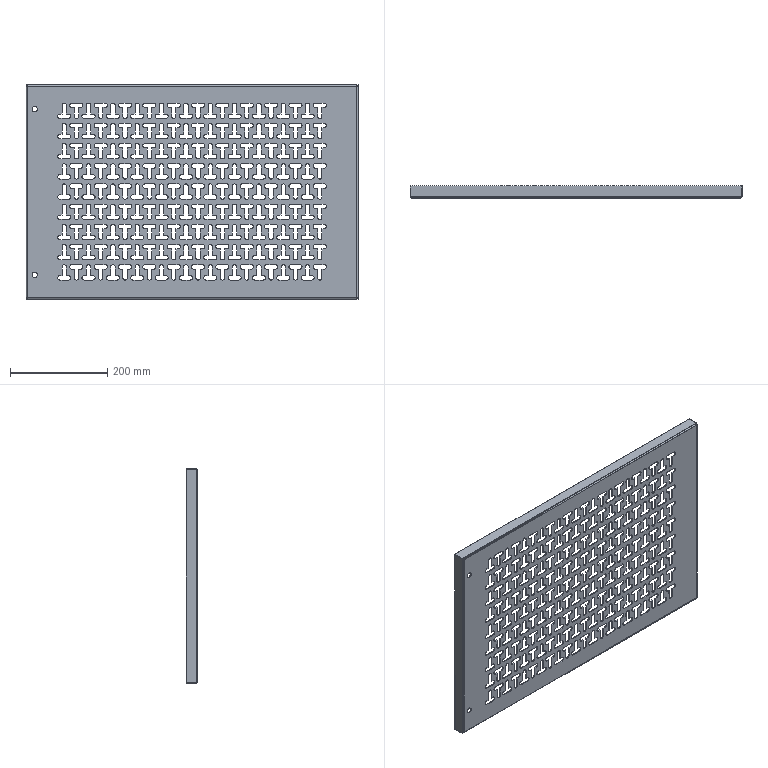Part | STEP file | 1 solid | 1848 faces | box 682 x 24 x 440 mm | volume 397013 mm3 | plane 1028 | cylinder 820 | commonest cylinder face diameters 9 x792 7 x16 3 x4 6 x4 11 x4